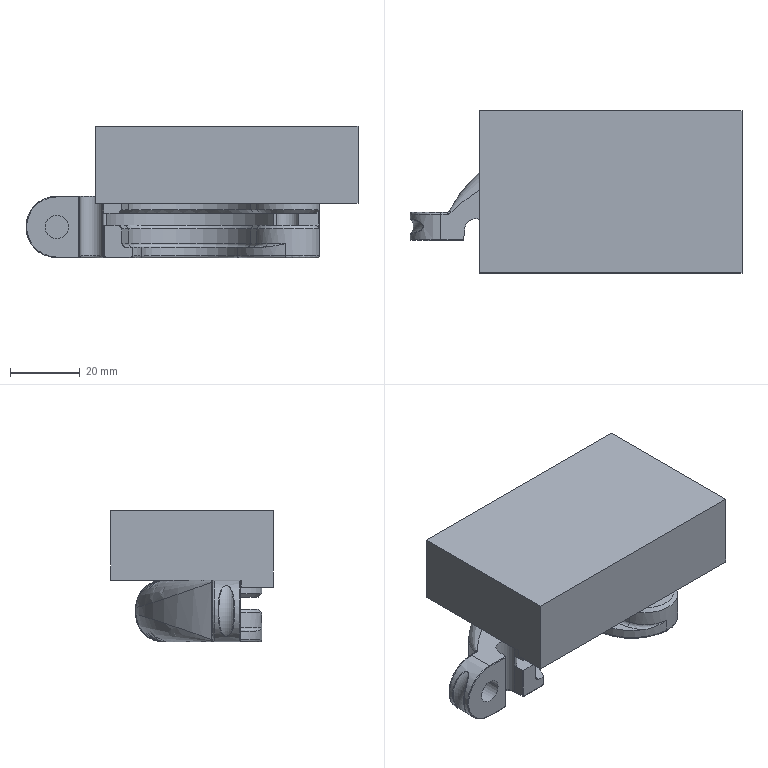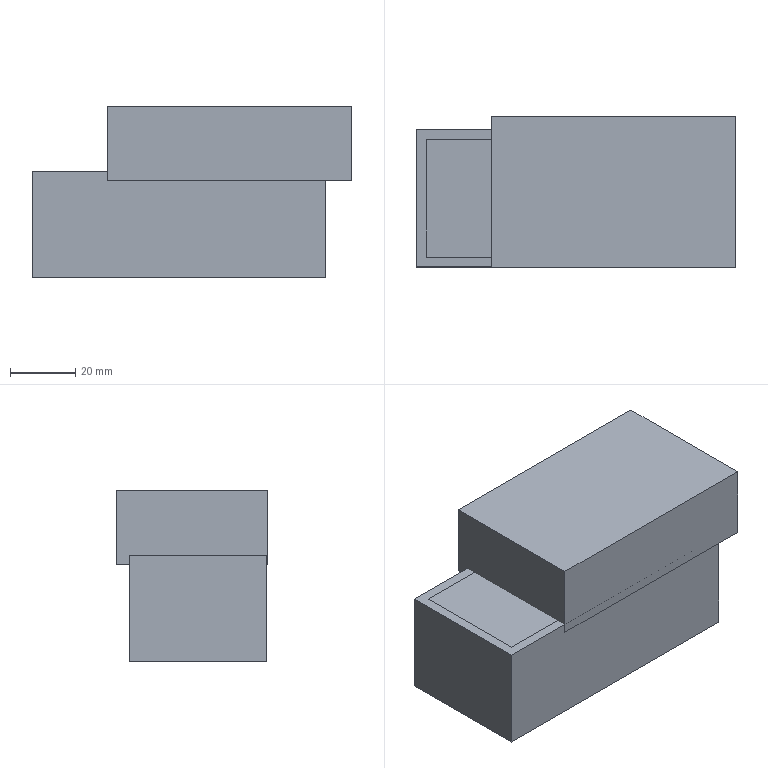CAM job | NX | 3+2 milling, drilling | part box 94.951 x 46.35 x 37.6 mm | stock box 97.95 x 46.35 x 52.6 mm
Tools:
number,name,description,diameter,corner_radius,flute_length,length,flutes
1,D63面刀,,63.0,0.0,50.0,75.0,2
19,D8开粗,,8.0,0.0,50.0,75.0,2
4,D6点钻,,6.0,0.0,50.0,75.0,2
5,D6.5钻头,,6.5,0.0,50.0,75.0,2
3,D5开粗,,5.0,0.0,50.0,75.0,2
23,D6R0.5,,6.0,0.5,50.0,75.0,2
6,T_CUTTER_1,,14.0,,3.0,25.0,4
12,倒角3.,,3.0,0.0,35.0,50.0,2
19,D16,,12.0,0.0,50.0,75.0,2
20,球刀3.,,3.0,1.5,50.0,75.0,2
6,D4.,,4.0,0.0,50.0,75.0,2
7,D5.,,5.0,0.0,50.0,75.0,2
15,D4,,4.0,0.0,50.0,75.0,2
Operations:
program,operation,operation_type,tool,method,geometry_group,spindle_rpm,surface_speed,feed_per_tooth,feed_cut,feed_plunge,cut_length_mm,path_length_mm,cut_time_min,machine_time_min
G54,FACE_MILLING,FaceMilling,D63面刀,MILL_ROUGH,WORKPIECE,4500.0,890.0,0.1667,1500.0,60.0,206.466,240.466,0.153,0.1564
G54,ADAPTIVE_MILLING,CavityMilling,D8开粗,MILL_ROUGH,WORKPIECE,6500.0,163.0,0.2692,3500.0,60.0,4354.341,4428.341,1.245,1.252
G54,CAVITY_MILL,CavityMilling,D8开粗,MILL_ROUGH,WORKPIECE,6500.0,163.0,0.2692,3500.0,60.0,2345.58,3604.584,0.7027,0.8588
G54,DRILLING,Operation,D6点钻,DRILL_METHOD,WORKPIECE,2000.0,37.0,0.0375,150.0,0.0,8.0,66.616,0.0533,0.0592
G54,DRILLING_COPY,Operation,D6.5钻头,DRILL_METHOD,WORKPIECE,2300.0,46.0,0.0326,150.0,0.0,22.0,84.0,0.1467,0.1529
G54,PLANAR_MILL,PlanarMilling,D5开粗,MILL_ROUGH,WORKPIECE,7000.0,109.0,0.0857,1200.0,60.0,303.581,400.504,0.298,0.3087
G54,PLANAR_MILL_COPY_1,PlanarMilling,D5开粗,MILL_FINISH,WORKPIECE,4500.0,70.0,0.0089,80.0,100.0,35.825,130.933,0.4478,0.4574
G54,PLANAR_MILL_COPY,PlanarMilling,D5开粗,MILL_ROUGH,WORKPIECE,6500.0,102.0,0.0385,500.0,60.0,30.113,69.713,0.0654,0.0694
G54,PLANAR_MILL_COPY_COPY,PlanarMilling,D5开粗,MILL_ROUGH,WORKPIECE,6500.0,102.0,0.0385,500.0,60.0,71.882,115.282,0.2253,0.2296
G54,PLANAR_MILL_COPY_COPY_COPY,PlanarMilling,D5开粗,MILL_ROUGH,WORKPIECE,5000.0,78.0,0.008,80.0,60.0,24.014,70.614,0.3186,0.3232
G54,PLANAR_MILL_COPY_COPY_1,PlanarMilling,D5开粗,MILL_FINISH,WORKPIECE,5000.0,78.0,0.008,80.0,100.0,31.266,70.866,0.3908,0.3948
G54,ZLEVEL_PROFILE_COPY,ZLevelMilling,D6R0.5,MILL_FINISH,WORKPIECE,6500.0,122.0,0.1923,2500.0,100.0,2920.369,3031.593,1.168,1.179
G54,PLANAR_MILL_1,PlanarMilling,T_CUTTER_1,MILL_ROUGH,WORKPIECE,2000.0,87.0,0.0375,300.0,60.0,118.349,164.549,0.4109,0.4156
G54,PLANAR_MILL_1_COPY,PlanarMilling,T_CUTTER_1,MILL_ROUGH,WORKPIECE,2000.0,87.0,0.0375,300.0,60.0,118.695,164.395,0.4125,0.4171
G54,PLANAR_MILL_1_COPY_COPY,PlanarMilling,T_CUTTER_1,MILL_ROUGH,WORKPIECE,2000.0,87.0,0.0375,300.0,60.0,118.695,165.395,0.4125,0.4172
G54,PLANAR_MILL_2,PlanarMilling,倒角3.,MILL_FINISH,WORKPIECE,5500.0,51.0,0.0909,1000.0,100.0,73.169,192.975,0.0732,0.0851
G54,PLANAR_MILL_2_COPY,PlanarMilling,倒角3.,MILL_FINISH,WORKPIECE,5500.0,51.0,0.0909,1000.0,100.0,27.85,65.45,0.0278,0.0316
G54,PLANAR_MILL_2_COPY_COPY,PlanarMilling,倒角3.,MILL_FINISH,WORKPIECE,5500.0,51.0,0.0909,1000.0,100.0,67.786,132.986,0.0678,0.0743
G58,PLANAR_MILL_3,PlanarMilling,D16,111,1,5500.0,138.0,0.2273,2500.0,100.0,8655.25,17808.2,3.462,4.377
G58,FACE_MILLING_2_COPY,FaceMilling,D63面刀,111,1,4500.0,890.0,0.0556,500.0,100.0,206.463,300.463,0.4129,0.4223
G58,ZLEVEL_PROFILE,ZLevelMilling,球刀3.,111,1,6500.0,122.0,0.1923,2500.0,100.0,4265.842,4366.854,1.706,1.716
G58,PLANAR_PROFILE,PlanarMilling,D4.,111,1,4500.0,56.0,0.0556,500.0,100.0,64.45,166.116,0.1289,0.1391
G58,PLANAR_PROFILE_COPY_COPY,PlanarMilling,D5.,111,1,5500.0,86.0,0.0273,300.0,100.0,13.292,120.892,0.0443,0.0551
G58,PLANAR_PROFILE_COPY,PlanarMilling,D5.,111,1,5500.0,86.0,0.0273,300.0,100.0,37.576,139.176,0.1253,0.1354
G58,PLANAR_PROFILE_COPY_COPY_COPY,PlanarMilling,D5.,111,1,5500.0,86.0,0.0273,300.0,100.0,13.802,121.402,0.046,0.0568
G58,PLANAR_MILL_4,PlanarMilling,倒角3.,METHOD,1,3500.0,32.0,0.1143,800.0,100.0,41.747,138.747,0.0522,0.0619
G58,PLANAR_MILL_4_COPY,PlanarMilling,倒角3.,METHOD,1,3500.0,32.0,0.1143,800.0,100.0,27.647,126.247,0.0346,0.0444
G,CAVITY_MILL_2,CavityMilling,D8开粗,111,WORKPIECE_1,5500.0,138.0,0.2273,2500.0,100.0,1176.156,2444.167,0.4705,0.5973
G,ZLEVEL_PROFILE_1,ZLevelMilling,D6R0.5,111,WORKPIECE_1,6500.0,122.0,0.1923,2500.0,100.0,2311.521,2355.911,0.9246,0.929
G,CONTOUR_AREA_COPY,SurfaceContour,球刀3.,METHOD,MCS,6500.0,61.0,0.1923,2500.0,100.0,8411.517,8457.995,3.365,3.369
FIXTURE,CAVITY_MILL_1_COPY,CavityMilling,D4,MILL_FINISH,WORKPIECE_2,5500.0,69.0,0.0727,800.0,100.0,7145.327,9946.618,8.932,9.212
FIXTURE,CAVITY_MILL_1_COPY_COPY,CavityMilling,D4,MILL_FINISH,WORKPIECE_2,5500.0,69.0,0.0727,800.0,100.0,160.379,300.609,0.2005,0.2145